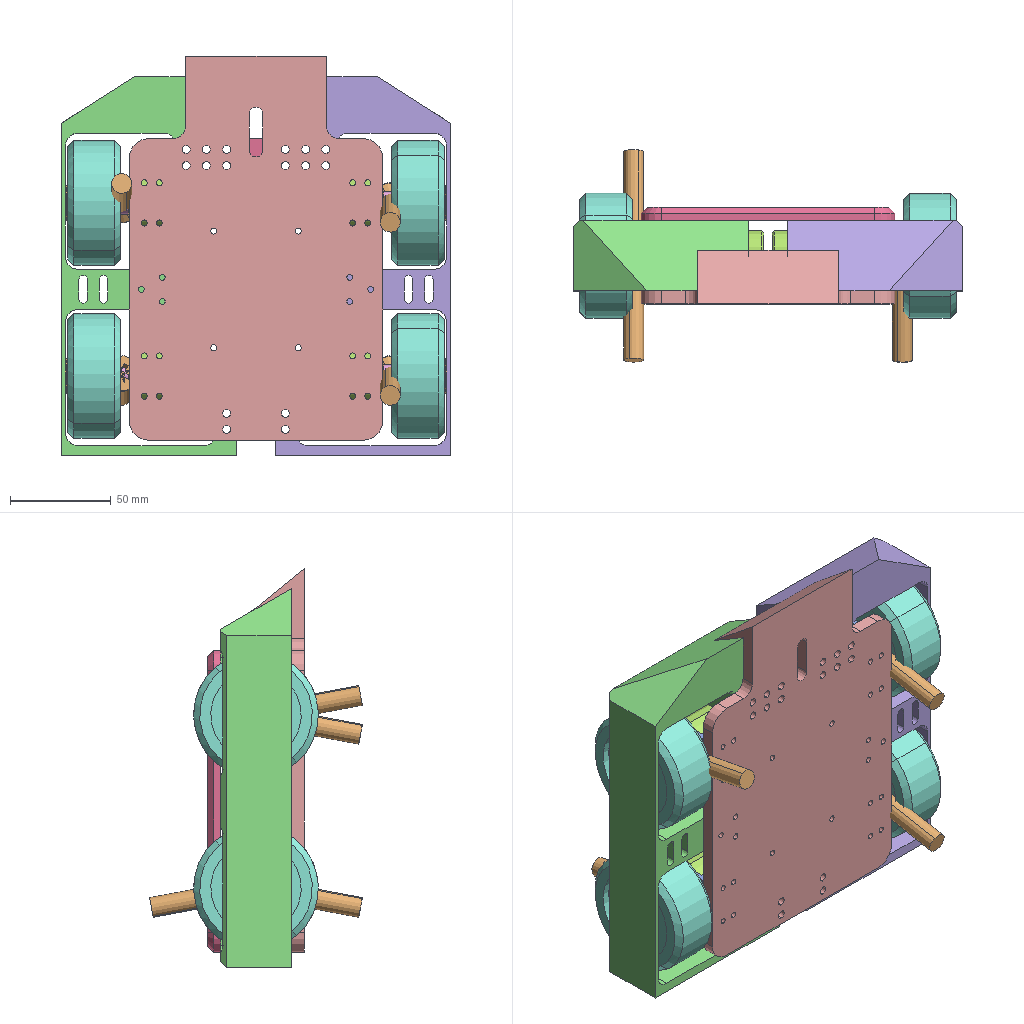Assembly | SolidWorks | 25 different items | 40 placed | box 193 x 106 x 198 mm
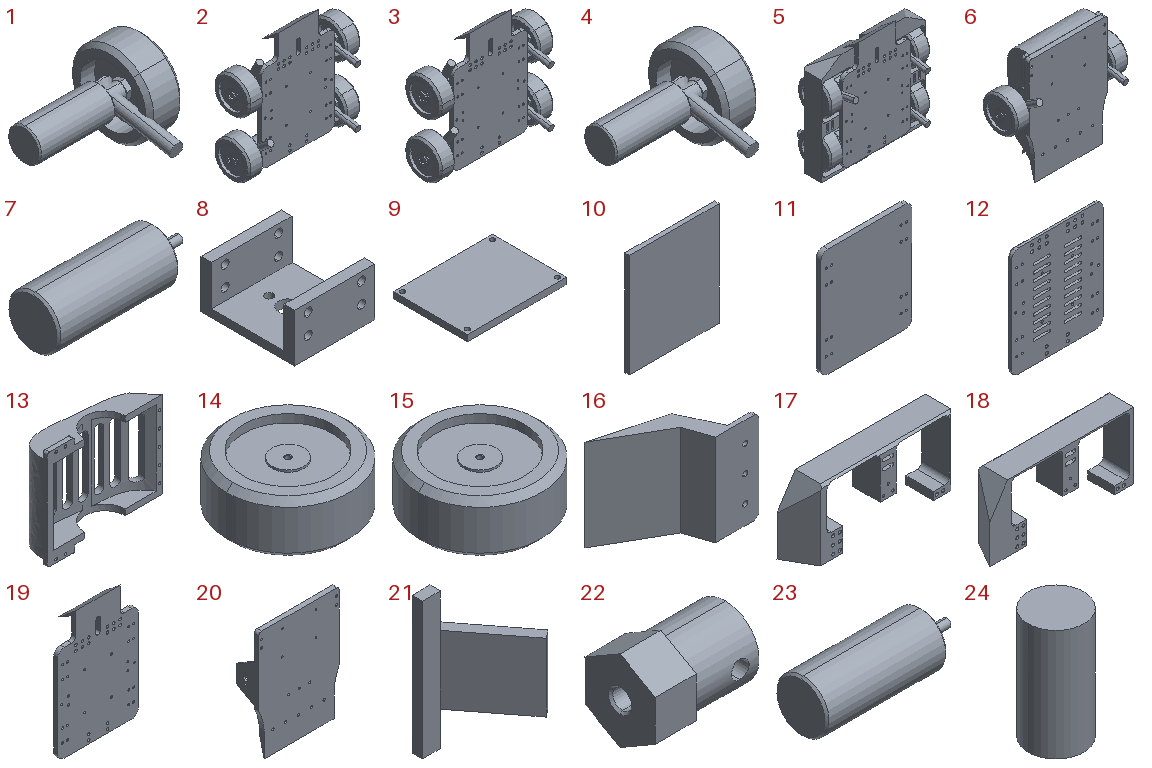Parts list (item | name | quantity | parent item | size | volume | features):
1 | (subassembly) | x1 | - | 93.4 x 83.824 x 62 mm | 93243 mm3 | features CompositeCurve 3
2 | (subassembly) | x1 | - | 196.8 x 83.824 x 200.07 mm | 523655 mm3 | -
3 | (subassembly) | x1 | - | 196.8 x 83.824 x 196.095 mm | 523655 mm3 | -
4 | (subassembly) | x4 | - | 93.4 x 83.824 x 62 mm | 93243 mm3 | features CompositeCurve 3
5 | (subassembly) | x1 | - | 193.215 x 105.647 x 198.21 mm | 922670 mm3 | -
6 | (subassembly) | x1 | - | 202.8 x 83.824 x 192.692 mm | 587716 mm3 | -
7 | - | x1 | - | 70 x 25 x 25 mm | 28507 mm3 | features ICE 3, Chamfer 2, Extrusion 1
8 | - | x4 | - | 30 x 35 x 18 mm | 6366 mm3 | features ICE 2, Extrusion 1, MirrorPattern 1
9 | - | x1 | - | 64 x 48 x 4 mm | 12175 mm3 | features Extrusion 1, ICE 1
10 | - | x1 | - | 130 x 6.5 x 150 mm | 126750 mm3 | features Extrusion 1
11 | - | x1 | - | 126 x 6.5 x 150 mm | 121557 mm3 | features MirrorPattern 2, Extrusion 1, Fillet 1, ICE 1
12 | - | x1 | - | 126 x 6.5 x 150 mm | 106751 mm3 | features ICE 6, MirrorPattern 5, Chamfer 1, Extrusion 1, Fillet 1
13 | - | x1 | - | 160.692 x 40.165 x 138 mm | 156504 mm3 | features ICE 5, Fillet 2, Extrusion 1, MirrorPattern 1, Shell 1
14 | - | x4 | in 4 | 62 x 62 x 26 mm | 52713 mm3 | features ICE 4, Chamfer 1, Extrusion 1, HoleWzd 1
15 | - | x1 | - | 62 x 62 x 26 mm | 52713 mm3 | features ICE 4, Chamfer 1, Extrusion 1, HoleWzd 1
16 | - | x1 | - | 77.912 x 41.912 x 63 mm | 38242 mm3 | features ICE 2, Extrusion 1, Fillet 1
17 | - | x1 | - | 188.207 x 35 x 87 mm | 133401 mm3 | features ICE 9, Fillet 4, MirrorPattern 3, Chamfer 1, Extrusion 1, LPattern 1
18 | - | x1 | - | 188.207 x 35 x 87 mm | 133399 mm3 | features ICE 9, Fillet 4, MirrorPattern 3, Chamfer 1, Extrusion 1, LPattern 1
19 | - | x1 | - | 126 x 26.5 x 190.71 mm | 150681 mm3 | features ICE 8, MirrorPattern 5, Fillet 2, Extrusion 1
20 | - | x1 | - | 138 x 38 x 192 mm | 194346 mm3 | features ICE 7, MirrorPattern 4, Extrusion 1, Fillet 1, Rib 1
21 | - | x1 | - | 42.25 x 40.996 x 80 mm | 16356 mm3 | features Extrusion 1, ICE 1, MirrorPattern 1
22 | - | x4 | in 4 | 18 x 12 x 13.856 mm | 1793 mm3 | features ICE 3, Extrusion 1, HoleWzd 1
23 | - | x4 | in 4 | 70 x 25 x 25 mm | 28507 mm3 | features ICE 3, Chamfer 2, Extrusion 1
24 | - | x1 | - | 20 x 20 x 40 mm | 12566 mm3 | features Extrusion 1
25 | cross recessed countersunk head screws gb1 | x1 | - | - | - | -
Mates (type | each side: item.copy, entity, surface, feature):
In the top assembly
Coincident | 19.1 face plane Boss-Extrude1 | 8.1 face plane Boss-Extrude1 | 2 times
Coincident | 19.1 face plane Boss-Extrude1 | 8.2 face plane Boss-Extrude1
Coincident | 19.1 face plane Boss-Extrude1 | 8.3 face plane Boss-Extrude1
Coincident | 19.1 face plane Boss-Extrude1 | 8.4 face plane Boss-Extrude1
Parallel | 19.1 face plane Boss-Extrude1 | 8.3 face plane Boss-Extrude1
Parallel | 19.1 face plane Boss-Extrude1 | 8.4 face plane Boss-Extrude1
Parallel | 19.1 face plane Boss-Extrude1 | 8.2 face plane Boss-Extrude1
Parallel | 19.1 face plane Boss-Extrude1 | 8.1 face plane Boss-Extrude1
Concentric | 8.1 face cylinder Boss-Extrude1 | 23.1 face cylinder Boss-Extrude2
Concentric | 8.2 face cylinder Boss-Extrude1 | 23.2 face cylinder Boss-Extrude2
Concentric | 8.3 face cylinder Boss-Extrude1 | 23.3 face cylinder Boss-Extrude2
Concentric | 8.4 face cylinder Boss-Extrude1 | 23.4 face cylinder Boss-Extrude2
Coincident | 8.2 face plane Boss-Extrude1 | 23.2 face plane Boss-Extrude1
Coincident | 8.3 face plane Boss-Extrude1 | 23.3 face plane Boss-Extrude1
Concentric | 8.3 face cylinder Boss-Extrude1 | 23.3 face cylinder Cut-Extrude1
Concentric | 8.2 face cylinder Boss-Extrude1 | 23.2 face cylinder Cut-Extrude1
Coincident | 8.4 face plane Boss-Extrude1 | 23.4 face plane Boss-Extrude1
Concentric | 8.4 face cylinder Boss-Extrude1 | 23.4 face cylinder Cut-Extrude1
Coincident | 8.1 face plane Boss-Extrude1 | 23.1 face plane Boss-Extrude1
Concentric | 8.1 face cylinder Boss-Extrude1 | 23.1 face cylinder Cut-Extrude1
Concentric | 19.1 face cylinder Mirror2 | 8.1 face cylinder Mirror1
Concentric | 19.1 face cylinder Cut-Extrude1 | 8.2 face cylinder Mirror1
Concentric | 19.1 face cylinder Mirror1 | 8.3 face cylinder Mirror1
Concentric | 19.1 face cylinder Mirror2 | 8.4 face cylinder Mirror1
Concentric | 19.1 face cylinder Mirror3 | 18.1 face cylinder Mirror1 | 2 times
Concentric | 19.1 face cylinder Cut-Extrude3 | 17.1 face cylinder Mirror1
Concentric | 19.1 face cylinder Cut-Extrude3 | 17.1 face cylinder Cut-Extrude1
Coincident | 18.1 face plane Boss-Extrude1 | 12.1 face plane Boss-Extrude1
Concentric | 18.1 face cylinder Mirror3 | 12.1 face cylinder Cut-Extrude4
Concentric | 17.1 face cylinder Cut-Extrude2 | 12.1 face cylinder Mirror5
Coincident | 19.1 face plane Boss-Extrude1 | 18.1 face plane Boss-Extrude1
Coincident | 17.1 face plane Boss-Extrude1 | 12.1 face plane Boss-Extrude1
In subassembly 4
Concentric | 23.5 face cylinder Boss-Extrude3 | 22.1 face cylinder Cut-Extrude1
DistanceDim | 23.5 face plane Boss-Extrude2 | 22.1 face plane Boss-Extrude2
Concentric | 22.1 face cylinder Boss-Extrude2 | 14.1 face cylinder Boss-Extrude1
Coincident | 22.1 face plane Boss-Extrude1 | 14.1 face plane Cut-Extrude2 | 2 times